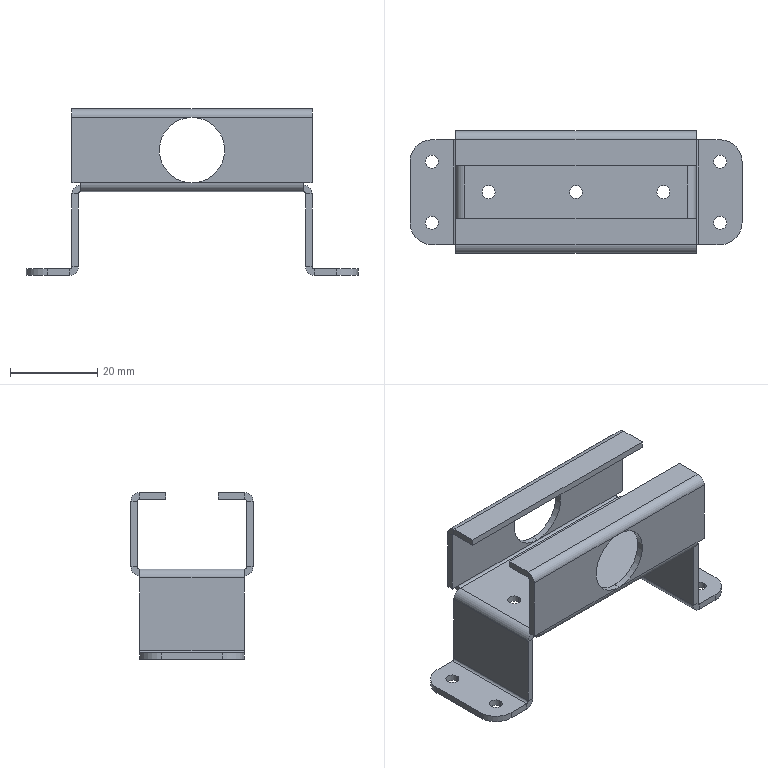Part | SolidWorks | features BaseBody 1 | 1 solid | 100 faces | box 76 x 28 x 38.15 mm | volume 7490 mm3 | plane 62 | cylinder 38 | commonest cylinder face diameters 3 x14 1 x8 4 x8 10 x4 15 x4